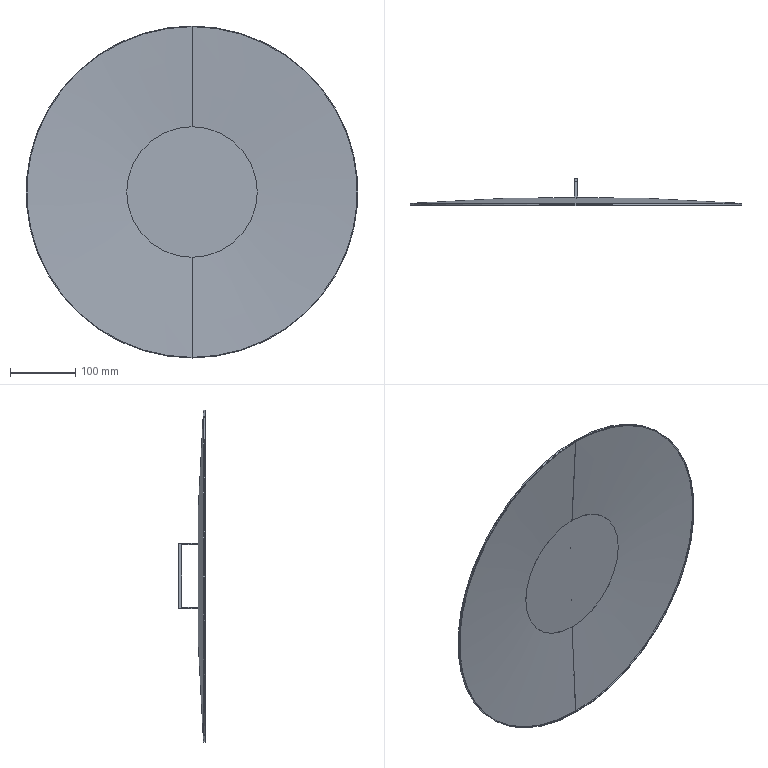Part | SolidWorks | features ICE 1, Revolution 1 | 1 solid | 19 faces | box 508 x 41 x 508 mm | volume 209061 mm3 | plane 11 | cylinder 4 | cone 4 | commonest cylinder face diameters 506 x2 508 x2